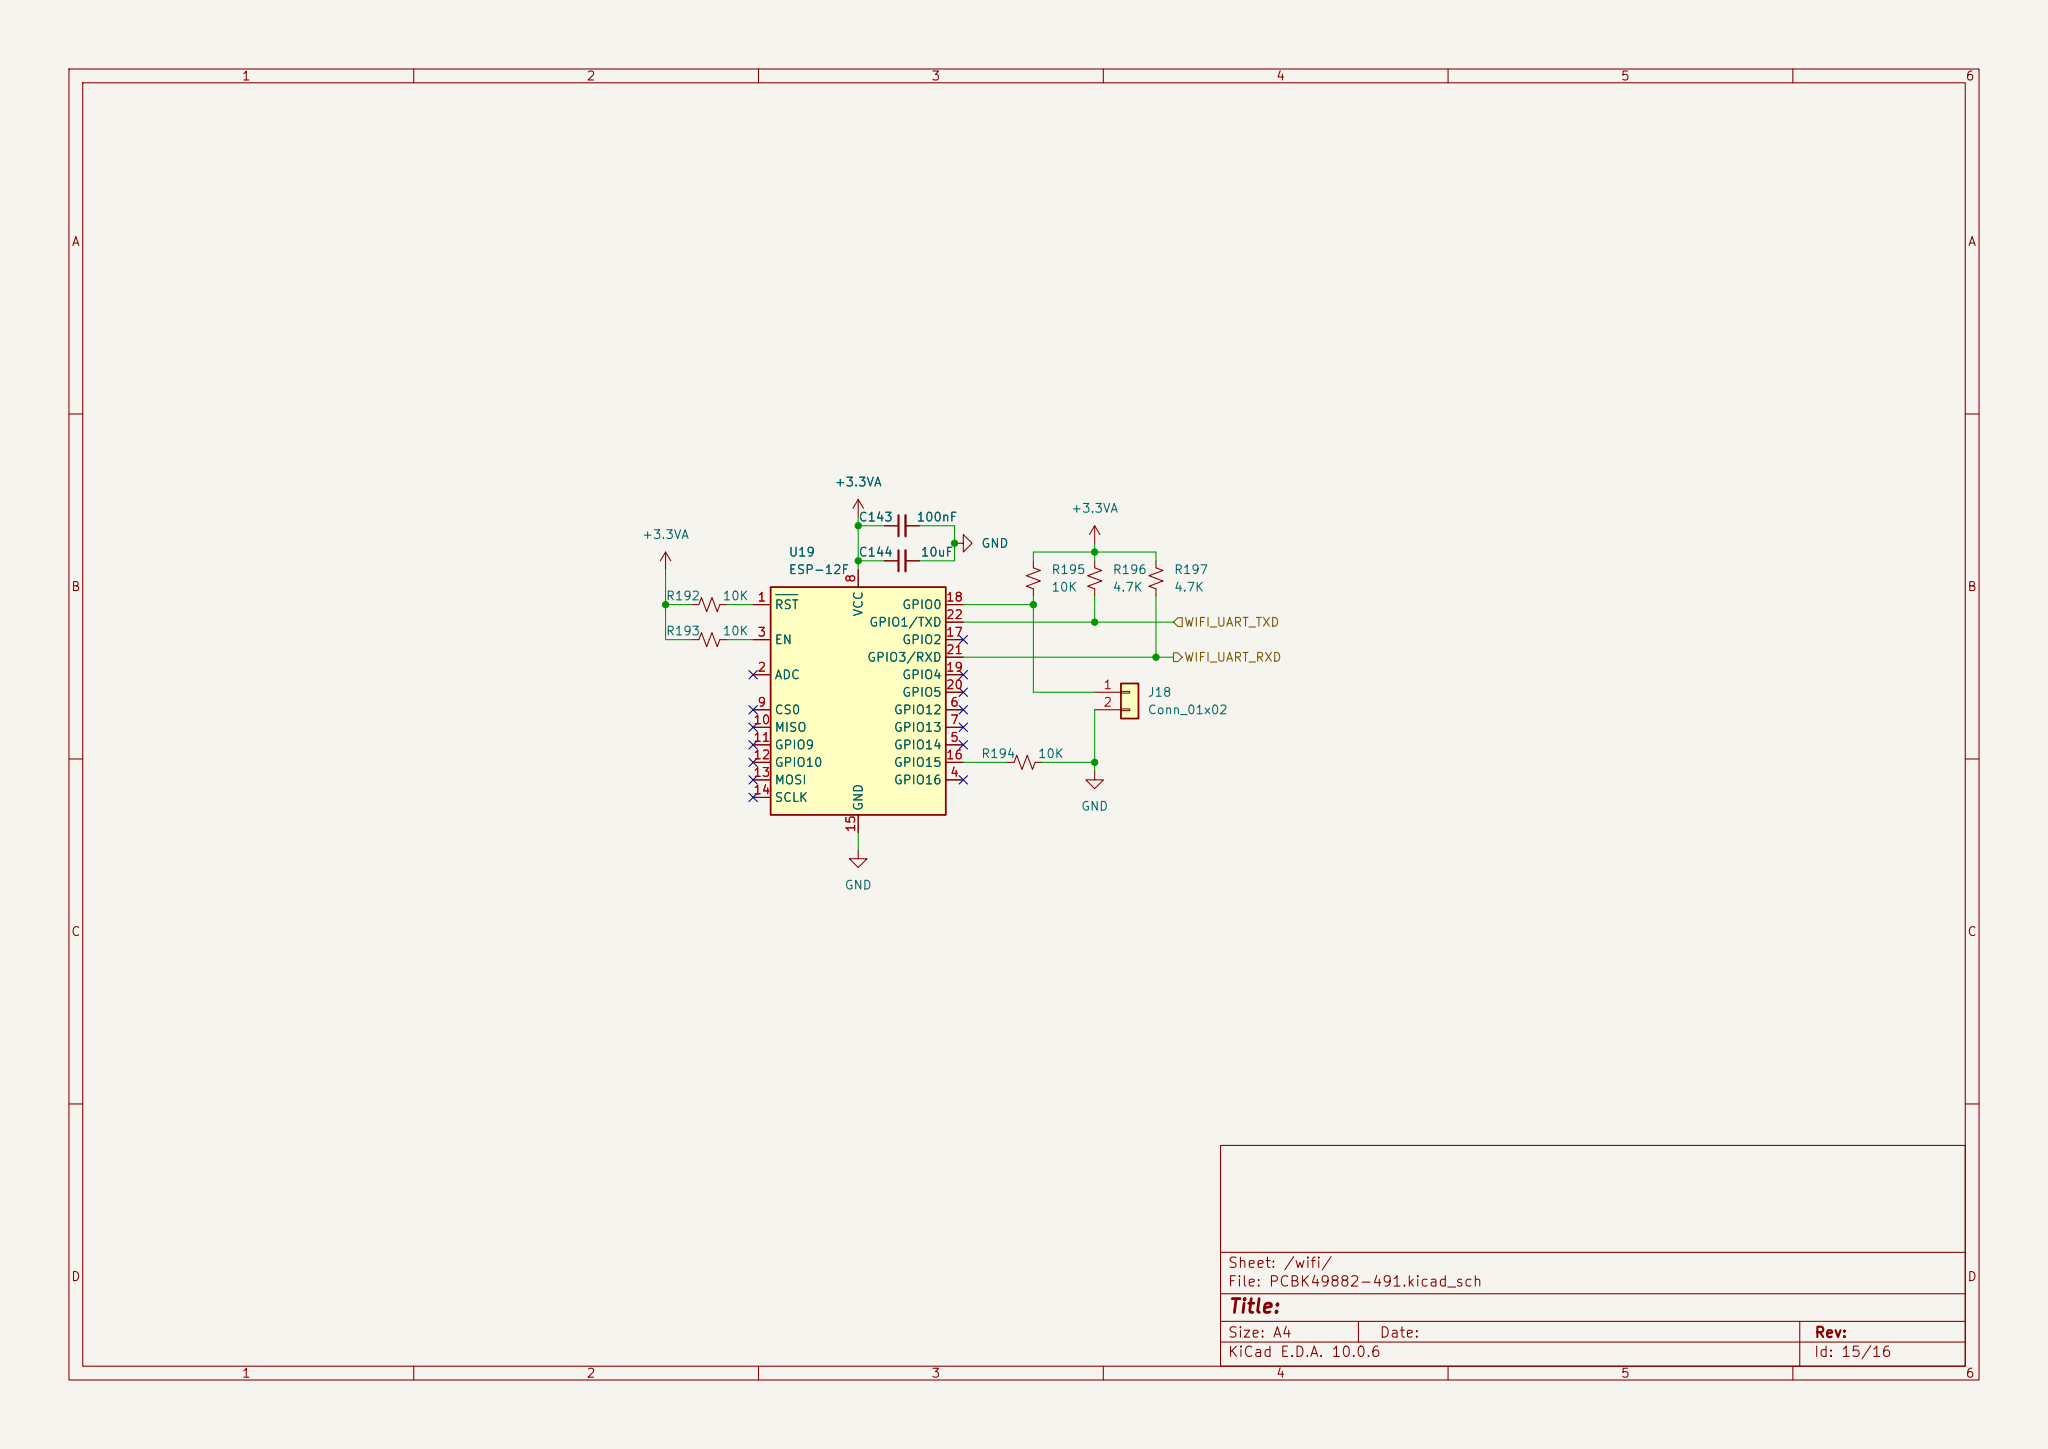Circuit board | KiCad | 536 parts | 438 nets | one sheet of the schematic
Parts on this sheet (reference | value | footprint):
C143 | 100nF | Capacitor_SMD:C_0603_1608Metric
C144 | 10uF | Capacitor_SMD:C_1210_3225Metric
J18 | Conn_01x02 | Connector_PinHeader_2.54mm:PinHeader_1x02_P2.54mm_Vertical
R192
R193
R194
R195
R196 | 4.7K | Resistor_SMD:R_0603_1608Metric
R197 | 4.7K | Resistor_SMD:R_0603_1608Metric
U19 | ESP-12F | RF_Module:ESP-12E
Nets of these parts (net: part-pin ...):
+3.3VA: C143-1 C144-1 R192-1 R193-1 R195-1 R196-1 R197-1 U19-8
/core_board_b2b/PB8{slash}UART4_RX{slash}FDCAN1_RX: R197-2 U19-21
/core_board_b2b/PB9{slash}UART4_TX{slash}FDCAN1_TX: R196-2 U19-22
GND: C143-2 C144-2 J18-2 R194-2 U19-15
Net-(J18-Pin_1): J18-1 R195-2 U19-18
Net-(U19-EN): R193-2 U19-3
Net-(U19-GPIO15): R194-1 U19-16
Net-(U19-~{RST}): R192-2 U19-1